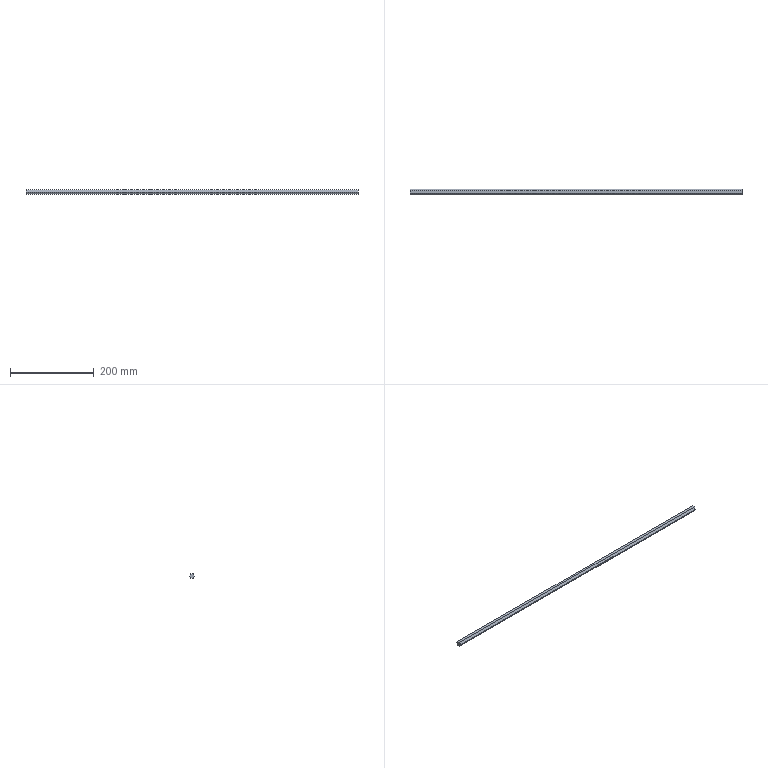Part | NX | features BREP 1 | 1 solid | 8 faces | box 792.5 x 12.702 x 11 mm | volume 83045 mm3 | plane 8
STEP:
#1=CARTESIAN_POINT('',(-396.25,-3.175,-5.5));
#2=VERTEX_POINT('',#1);
#3=CARTESIAN_POINT('',(-396.25,3.175,-5.5));
#4=VERTEX_POINT('',#3);
#5=CARTESIAN_POINT('',(-396.25,-3.175,-5.5));
#6=DIRECTION('',(0.,1.,0.));
#7=VECTOR('',#6,1000.);
#8=LINE('',#5,#7);
#9=EDGE_CURVE('',#2,#4,#8,.T.);
#10=ORIENTED_EDGE('',*,*,#9,.F.);
#11=CARTESIAN_POINT('',(-396.25,-6.351,0.));
#12=VERTEX_POINT('',#11);
#13=CARTESIAN_POINT('',(-396.25,-6.351,0.));
#14=DIRECTION('',(0.,0.5,-0.866));
#15=VECTOR('',#14,1000.);
#16=LINE('',#13,#15);
#17=EDGE_CURVE('',#12,#2,#16,.T.);
#18=ORIENTED_EDGE('',*,*,#17,.F.);
#19=CARTESIAN_POINT('',(-396.25,-3.175,5.5));
#20=VERTEX_POINT('',#19);
#21=CARTESIAN_POINT('',(-396.25,-3.175,5.5));
#22=DIRECTION('',(0.,-0.5,-0.866));
#23=VECTOR('',#22,1000.);
#24=LINE('',#21,#23);
#25=EDGE_CURVE('',#20,#12,#24,.T.);
#26=ORIENTED_EDGE('',*,*,#25,.F.);
#27=CARTESIAN_POINT('',(-396.25,3.175,5.5));
#28=VERTEX_POINT('',#27);
#29=CARTESIAN_POINT('',(-396.25,3.175,5.5));
#30=DIRECTION('',(0.,-1.,0.));
#31=VECTOR('',#30,1000.);
#32=LINE('',#29,#31);
#33=EDGE_CURVE('',#28,#20,#32,.T.);
#34=ORIENTED_EDGE('',*,*,#33,.F.);
#35=CARTESIAN_POINT('',(-396.25,6.351,0.));
#36=VERTEX_POINT('',#35);
#37=CARTESIAN_POINT('',(-396.25,6.351,0.));
#38=DIRECTION('',(0.,-0.5,0.866));
#39=VECTOR('',#38,1000.);
#40=LINE('',#37,#39);
#41=EDGE_CURVE('',#36,#28,#40,.T.);
#42=ORIENTED_EDGE('',*,*,#41,.F.);
#43=CARTESIAN_POINT('',(-396.25,3.175,-5.5));
#44=DIRECTION('',(0.,0.5,0.866));
#45=VECTOR('',#44,1000.);
#46=LINE('',#43,#45);
#47=EDGE_CURVE('',#4,#36,#46,.T.);
#48=ORIENTED_EDGE('',*,*,#47,.F.);
#49=EDGE_LOOP('',(#10,#18,#26,#34,#42,#48));
#50=FACE_BOUND('',#49,.T.);
#51=CARTESIAN_POINT('',(-396.25,0.,0.));
#52=DIRECTION('',(1.,0.,0.));
#53=DIRECTION('',(0.,1.,0.));
#54=AXIS2_PLACEMENT_3D('',#51,#52,#53);
#55=PLANE('',#54);
#56=ADVANCED_FACE('',(#50),#55,.F.);
#57=CARTESIAN_POINT('',(396.25,6.351,0.));
#58=VERTEX_POINT('',#57);
#59=CARTESIAN_POINT('',(-396.25,6.351,0.));
#60=DIRECTION('',(1.,0.,0.));
#61=VECTOR('',#60,1000.);
#62=LINE('',#59,#61);
#63=EDGE_CURVE('',#36,#58,#62,.T.);
#64=ORIENTED_EDGE('',*,*,#63,.T.);
#65=CARTESIAN_POINT('',(396.25,3.175,-5.5));
#66=VERTEX_POINT('',#65);
#67=CARTESIAN_POINT('',(396.25,3.175,-5.5));
#68=DIRECTION('',(0.,0.5,0.866));
#69=VECTOR('',#68,1000.);
#70=LINE('',#67,#69);
#71=EDGE_CURVE('',#66,#58,#70,.T.);
#72=ORIENTED_EDGE('',*,*,#71,.F.);
#73=CARTESIAN_POINT('',(-396.25,3.175,-5.5));
#74=DIRECTION('',(1.,0.,0.));
#75=VECTOR('',#74,1000.);
#76=LINE('',#73,#75);
#77=EDGE_CURVE('',#4,#66,#76,.T.);
#78=ORIENTED_EDGE('',*,*,#77,.F.);
#79=ORIENTED_EDGE('',*,*,#47,.T.);
#80=EDGE_LOOP('',(#64,#72,#78,#79));
#81=FACE_BOUND('',#80,.T.);
#82=CARTESIAN_POINT('',(-396.25,3.175,-5.5));
#83=DIRECTION('',(0.,0.866,-0.5));
#84=DIRECTION('',(-1.,0.,0.));
#85=AXIS2_PLACEMENT_3D('',#82,#83,#84);
#86=PLANE('',#85);
#87=ADVANCED_FACE('',(#81),#86,.T.);
#88=ORIENTED_EDGE('',*,*,#77,.T.);
#89=CARTESIAN_POINT('',(396.25,-3.175,-5.5));
#90=VERTEX_POINT('',#89);
#91=CARTESIAN_POINT('',(396.25,-3.175,-5.5));
#92=DIRECTION('',(0.,1.,0.));
#93=VECTOR('',#92,1000.);
#94=LINE('',#91,#93);
#95=EDGE_CURVE('',#90,#66,#94,.T.);
#96=ORIENTED_EDGE('',*,*,#95,.F.);
#97=CARTESIAN_POINT('',(-396.25,-3.175,-5.5));
#98=DIRECTION('',(1.,0.,0.));
#99=VECTOR('',#98,1000.);
#100=LINE('',#97,#99);
#101=EDGE_CURVE('',#2,#90,#100,.T.);
#102=ORIENTED_EDGE('',*,*,#101,.F.);
#103=ORIENTED_EDGE('',*,*,#9,.T.);
#104=EDGE_LOOP('',(#88,#96,#102,#103));
#105=FACE_BOUND('',#104,.T.);
#106=CARTESIAN_POINT('',(-396.25,-3.175,-5.5));
#107=DIRECTION('',(0.,0.,-1.));
#108=DIRECTION('',(0.,-1.,0.));
#109=AXIS2_PLACEMENT_3D('',#106,#107,#108);
#110=PLANE('',#109);
#111=ADVANCED_FACE('',(#105),#110,.T.);
#112=ORIENTED_EDGE('',*,*,#101,.T.);
#113=CARTESIAN_POINT('',(396.25,-6.351,0.));
#114=VERTEX_POINT('',#113);
#115=CARTESIAN_POINT('',(396.25,-6.351,0.));
#116=DIRECTION('',(0.,0.5,-0.866));
#117=VECTOR('',#116,1000.);
#118=LINE('',#115,#117);
#119=EDGE_CURVE('',#114,#90,#118,.T.);
#120=ORIENTED_EDGE('',*,*,#119,.F.);
#121=CARTESIAN_POINT('',(-396.25,-6.351,0.));
#122=DIRECTION('',(1.,0.,0.));
#123=VECTOR('',#122,1000.);
#124=LINE('',#121,#123);
#125=EDGE_CURVE('',#12,#114,#124,.T.);
#126=ORIENTED_EDGE('',*,*,#125,.F.);
#127=ORIENTED_EDGE('',*,*,#17,.T.);
#128=EDGE_LOOP('',(#112,#120,#126,#127));
#129=FACE_BOUND('',#128,.T.);
#130=CARTESIAN_POINT('',(-396.25,-6.351,0.));
#131=DIRECTION('',(0.,-0.866,-0.5));
#132=DIRECTION('',(0.,0.5,-0.866));
#133=AXIS2_PLACEMENT_3D('',#130,#131,#132);
#134=PLANE('',#133);
#135=ADVANCED_FACE('',(#129),#134,.T.);
#136=ORIENTED_EDGE('',*,*,#125,.T.);
#137=CARTESIAN_POINT('',(396.25,-3.175,5.5));
#138=VERTEX_POINT('',#137);
#139=CARTESIAN_POINT('',(396.25,-3.175,5.5));
#140=DIRECTION('',(0.,-0.5,-0.866));
#141=VECTOR('',#140,1000.);
#142=LINE('',#139,#141);
#143=EDGE_CURVE('',#138,#114,#142,.T.);
#144=ORIENTED_EDGE('',*,*,#143,.F.);
#145=CARTESIAN_POINT('',(-396.25,-3.175,5.5));
#146=DIRECTION('',(1.,0.,0.));
#147=VECTOR('',#146,1000.);
#148=LINE('',#145,#147);
#149=EDGE_CURVE('',#20,#138,#148,.T.);
#150=ORIENTED_EDGE('',*,*,#149,.F.);
#151=ORIENTED_EDGE('',*,*,#25,.T.);
#152=EDGE_LOOP('',(#136,#144,#150,#151));
#153=FACE_BOUND('',#152,.T.);
#154=CARTESIAN_POINT('',(-396.25,-3.175,5.5));
#155=DIRECTION('',(0.,-0.866,0.5));
#156=DIRECTION('',(-1.,0.,0.));
#157=AXIS2_PLACEMENT_3D('',#154,#155,#156);
#158=PLANE('',#157);
#159=ADVANCED_FACE('',(#153),#158,.T.);
#160=ORIENTED_EDGE('',*,*,#149,.T.);
#161=CARTESIAN_POINT('',(396.25,3.175,5.5));
#162=VERTEX_POINT('',#161);
#163=CARTESIAN_POINT('',(396.25,3.175,5.5));
#164=DIRECTION('',(0.,-1.,0.));
#165=VECTOR('',#164,1000.);
#166=LINE('',#163,#165);
#167=EDGE_CURVE('',#162,#138,#166,.T.);
#168=ORIENTED_EDGE('',*,*,#167,.F.);
#169=CARTESIAN_POINT('',(-396.25,3.175,5.5));
#170=DIRECTION('',(1.,0.,0.));
#171=VECTOR('',#170,1000.);
#172=LINE('',#169,#171);
#173=EDGE_CURVE('',#28,#162,#172,.T.);
#174=ORIENTED_EDGE('',*,*,#173,.F.);
#175=ORIENTED_EDGE('',*,*,#33,.T.);
#176=EDGE_LOOP('',(#160,#168,#174,#175));
#177=FACE_BOUND('',#176,.T.);
#178=CARTESIAN_POINT('',(-396.25,3.175,5.5));
#179=DIRECTION('',(0.,0.,1.));
#180=DIRECTION('',(1.,0.,0.));
#181=AXIS2_PLACEMENT_3D('',#178,#179,#180);
#182=PLANE('',#181);
#183=ADVANCED_FACE('',(#177),#182,.T.);
#184=ORIENTED_EDGE('',*,*,#173,.T.);
#185=CARTESIAN_POINT('',(396.25,6.351,0.));
#186=DIRECTION('',(0.,-0.5,0.866));
#187=VECTOR('',#186,1000.);
#188=LINE('',#185,#187);
#189=EDGE_CURVE('',#58,#162,#188,.T.);
#190=ORIENTED_EDGE('',*,*,#189,.F.);
#191=ORIENTED_EDGE('',*,*,#63,.F.);
#192=ORIENTED_EDGE('',*,*,#41,.T.);
#193=EDGE_LOOP('',(#184,#190,#191,#192));
#194=FACE_BOUND('',#193,.T.);
#195=CARTESIAN_POINT('',(-396.25,6.351,0.));
#196=DIRECTION('',(0.,0.866,0.5));
#197=DIRECTION('',(1.,0.,0.));
#198=AXIS2_PLACEMENT_3D('',#195,#196,#197);
#199=PLANE('',#198);
#200=ADVANCED_FACE('',(#194),#199,.T.);
#201=ORIENTED_EDGE('',*,*,#189,.T.);
#202=ORIENTED_EDGE('',*,*,#167,.T.);
#203=ORIENTED_EDGE('',*,*,#143,.T.);
#204=ORIENTED_EDGE('',*,*,#119,.T.);
#205=ORIENTED_EDGE('',*,*,#95,.T.);
#206=ORIENTED_EDGE('',*,*,#71,.T.);
#207=EDGE_LOOP('',(#201,#202,#203,#204,#205,#206));
#208=FACE_BOUND('',#207,.T.);
#209=CARTESIAN_POINT('',(396.25,0.,0.));
#210=DIRECTION('',(1.,0.,0.));
#211=DIRECTION('',(0.,1.,0.));
#212=AXIS2_PLACEMENT_3D('',#209,#210,#211);
#213=PLANE('',#212);
#214=ADVANCED_FACE('',(#208),#213,.T.);
#215=CLOSED_SHELL('',(#56,#87,#111,#135,#159,#183,#200,#214));
#216=MANIFOLD_SOLID_BREP('',#215);
#217=(LENGTH_UNIT()NAMED_UNIT(*)SI_UNIT(.MILLI.,.METRE.));
#218=UNCERTAINTY_MEASURE_WITH_UNIT(LENGTH_MEASURE(0.00001),#217,'','');
#219=(NAMED_UNIT(*)PLANE_ANGLE_UNIT()SI_UNIT($,.RADIAN.));
#220=(NAMED_UNIT(*)SI_UNIT($,.STERADIAN.)SOLID_ANGLE_UNIT());
#221=(GEOMETRIC_REPRESENTATION_CONTEXT(3)GLOBAL_UNCERTAINTY_ASSIGNED_CONTEXT((#218))GLOBAL_UNIT_ASSIGNED_CONTEXT((#217,#219,#220))REPRESENTATION_CONTEXT('',''));
#222=ADVANCED_BREP_SHAPE_REPRESENTATION('',(#216),#221);